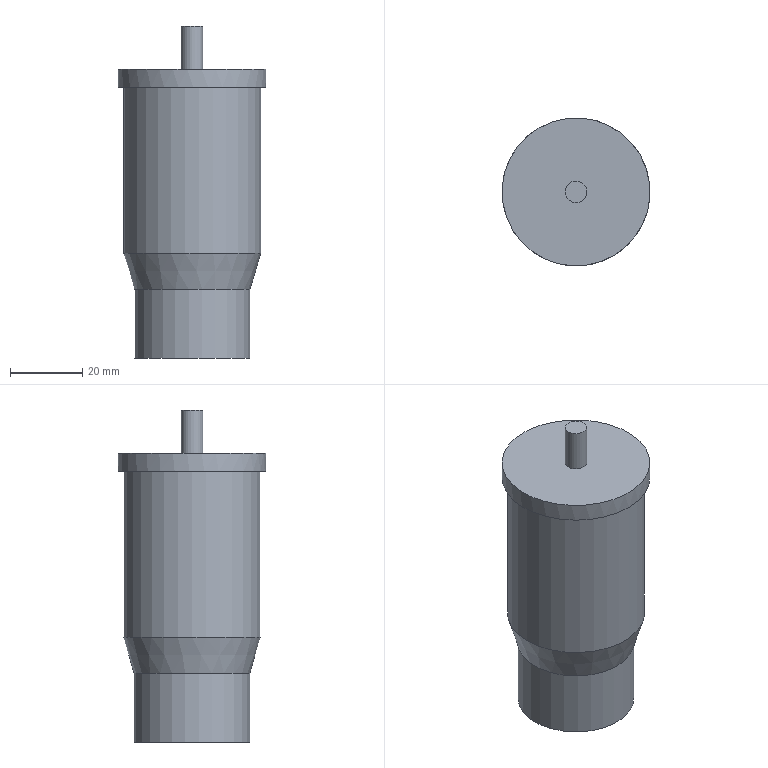Part | NX | features solid 2 | 1 solid | 9 faces | box 41 x 41 x 92 mm | volume 84158 mm3 | plane 4 | cylinder 4 | cone 1 | commonest cylinder face diameters 6 x1 32.1 x1 38 x1 41 x1
STEP:
#1=CARTESIAN_POINT('',(799.065,-200.244,51.));
#2=VERTEX_POINT('',#1);
#3=CARTESIAN_POINT('',(807.09,-214.144,51.));
#4=DIRECTION('',(0.,0.,-1.));
#5=DIRECTION('',(-0.5,0.866,0.));
#6=AXIS2_PLACEMENT_3D('',#3,#4,#5);
#7=CIRCLE('',#6,16.05);
#8=EDGE_CURVE('',#2,#2,#7,.T.);
#9=ORIENTED_EDGE('',*,*,#8,.T.);
#10=EDGE_LOOP('',(#9));
#11=FACE_BOUND('',#10,.T.);
#12=CARTESIAN_POINT('',(807.09,-214.144,51.));
#13=DIRECTION('',(0.,0.,-1.));
#14=DIRECTION('',(0.5,-0.866,0.));
#15=AXIS2_PLACEMENT_3D('',#12,#13,#14);
#16=PLANE('',#15);
#17=ADVANCED_FACE('',(#11),#16,.T.);
#18=CARTESIAN_POINT('',(799.065,-200.244,70.));
#19=VERTEX_POINT('',#18);
#20=CARTESIAN_POINT('',(807.09,-214.144,70.));
#21=DIRECTION('',(0.,0.,-1.));
#22=DIRECTION('',(-0.5,0.866,0.));
#23=AXIS2_PLACEMENT_3D('',#20,#21,#22);
#24=CIRCLE('',#23,16.05);
#25=EDGE_CURVE('',#19,#19,#24,.T.);
#26=ORIENTED_EDGE('',*,*,#25,.T.);
#27=EDGE_LOOP('',(#26));
#28=FACE_BOUND('',#27,.T.);
#29=ORIENTED_EDGE('',*,*,#8,.F.);
#30=EDGE_LOOP('',(#29));
#31=FACE_BOUND('',#30,.T.);
#32=CARTESIAN_POINT('',(807.09,-214.144,51.));
#33=DIRECTION('',(0.,0.,1.));
#34=DIRECTION('',(-0.5,0.866,0.));
#35=AXIS2_PLACEMENT_3D('',#32,#33,#34);
#36=CYLINDRICAL_SURFACE('',#35,16.05);
#37=ADVANCED_FACE('',(#28,#31),#36,.T.);
#38=ORIENTED_EDGE('',*,*,#25,.F.);
#39=EDGE_LOOP('',(#38));
#40=FACE_BOUND('',#39,.T.);
#41=CARTESIAN_POINT('',(797.59,-197.689,80.));
#42=VERTEX_POINT('',#41);
#43=CARTESIAN_POINT('',(807.09,-214.144,80.));
#44=DIRECTION('',(0.,0.,-1.));
#45=DIRECTION('',(-0.5,0.866,0.));
#46=AXIS2_PLACEMENT_3D('',#43,#44,#45);
#47=CIRCLE('',#46,19.);
#48=EDGE_CURVE('',#42,#42,#47,.T.);
#49=ORIENTED_EDGE('',*,*,#48,.T.);
#50=EDGE_LOOP('',(#49));
#51=FACE_BOUND('',#50,.T.);
#52=CARTESIAN_POINT('',(807.09,-214.144,70.));
#53=DIRECTION('',(0.,0.,1.));
#54=DIRECTION('',(-0.5,0.866,0.));
#55=AXIS2_PLACEMENT_3D('',#52,#53,#54);
#56=CONICAL_SURFACE('',#55,16.05,0.2869);
#57=ADVANCED_FACE('',(#40,#51),#56,.T.);
#58=CARTESIAN_POINT('',(816.59,-230.598,126.));
#59=VERTEX_POINT('',#58);
#60=CARTESIAN_POINT('',(807.09,-214.144,126.));
#61=DIRECTION('',(0.,0.,1.));
#62=DIRECTION('',(0.5,-0.866,0.));
#63=AXIS2_PLACEMENT_3D('',#60,#61,#62);
#64=CIRCLE('',#63,19.);
#65=EDGE_CURVE('',#59,#59,#64,.F.);
#66=ORIENTED_EDGE('',*,*,#65,.T.);
#67=EDGE_LOOP('',(#66));
#68=FACE_BOUND('',#67,.T.);
#69=ORIENTED_EDGE('',*,*,#48,.F.);
#70=EDGE_LOOP('',(#69));
#71=FACE_BOUND('',#70,.T.);
#72=CARTESIAN_POINT('',(807.09,-214.144,80.));
#73=DIRECTION('',(0.,0.,1.));
#74=DIRECTION('',(-0.5,0.866,0.));
#75=AXIS2_PLACEMENT_3D('',#72,#73,#74);
#76=CYLINDRICAL_SURFACE('',#75,19.);
#77=ADVANCED_FACE('',(#68,#71),#76,.T.);
#78=CARTESIAN_POINT('',(805.59,-211.545,131.));
#79=VERTEX_POINT('',#78);
#80=CARTESIAN_POINT('',(807.09,-214.144,131.));
#81=DIRECTION('',(0.,0.,-1.));
#82=DIRECTION('',(-0.5,0.866,0.));
#83=AXIS2_PLACEMENT_3D('',#80,#81,#82);
#84=CIRCLE('',#83,3.);
#85=EDGE_CURVE('',#79,#79,#84,.T.);
#86=ORIENTED_EDGE('',*,*,#85,.T.);
#87=EDGE_LOOP('',(#86));
#88=FACE_BOUND('',#87,.T.);
#89=CARTESIAN_POINT('',(817.34,-231.897,131.));
#90=VERTEX_POINT('',#89);
#91=CARTESIAN_POINT('',(807.09,-214.144,131.));
#92=DIRECTION('',(0.,0.,1.));
#93=DIRECTION('',(0.5,-0.866,0.));
#94=AXIS2_PLACEMENT_3D('',#91,#92,#93);
#95=CIRCLE('',#94,20.5);
#96=EDGE_CURVE('',#90,#90,#95,.T.);
#97=ORIENTED_EDGE('',*,*,#96,.T.);
#98=EDGE_LOOP('',(#97));
#99=FACE_BOUND('',#98,.T.);
#100=CARTESIAN_POINT('',(807.09,-214.144,131.));
#101=DIRECTION('',(0.,0.,1.));
#102=DIRECTION('',(-0.5,0.866,0.));
#103=AXIS2_PLACEMENT_3D('',#100,#101,#102);
#104=PLANE('',#103);
#105=ADVANCED_FACE('',(#88,#99),#104,.T.);
#106=ORIENTED_EDGE('',*,*,#65,.F.);
#107=EDGE_LOOP('',(#106));
#108=FACE_BOUND('',#107,.T.);
#109=CARTESIAN_POINT('',(796.84,-196.39,126.));
#110=VERTEX_POINT('',#109);
#111=CARTESIAN_POINT('',(807.09,-214.144,126.));
#112=DIRECTION('',(0.,0.,-1.));
#113=DIRECTION('',(-0.5,0.866,0.));
#114=AXIS2_PLACEMENT_3D('',#111,#112,#113);
#115=CIRCLE('',#114,20.5);
#116=EDGE_CURVE('',#110,#110,#115,.T.);
#117=ORIENTED_EDGE('',*,*,#116,.T.);
#118=EDGE_LOOP('',(#117));
#119=FACE_BOUND('',#118,.T.);
#120=CARTESIAN_POINT('',(807.09,-214.144,126.));
#121=DIRECTION('',(0.,0.,-1.));
#122=DIRECTION('',(0.5,-0.866,0.));
#123=AXIS2_PLACEMENT_3D('',#120,#121,#122);
#124=PLANE('',#123);
#125=ADVANCED_FACE('',(#108,#119),#124,.T.);
#126=ORIENTED_EDGE('',*,*,#96,.F.);
#127=EDGE_LOOP('',(#126));
#128=FACE_BOUND('',#127,.T.);
#129=ORIENTED_EDGE('',*,*,#116,.F.);
#130=EDGE_LOOP('',(#129));
#131=FACE_BOUND('',#130,.T.);
#132=CARTESIAN_POINT('',(807.09,-214.144,136.));
#133=DIRECTION('',(0.,0.,1.));
#134=DIRECTION('',(-0.5,0.866,0.));
#135=AXIS2_PLACEMENT_3D('',#132,#133,#134);
#136=CYLINDRICAL_SURFACE('',#135,20.5);
#137=ADVANCED_FACE('',(#128,#131),#136,.T.);
#138=CARTESIAN_POINT('',(808.59,-216.742,143.));
#139=VERTEX_POINT('',#138);
#140=CARTESIAN_POINT('',(807.09,-214.144,143.));
#141=DIRECTION('',(0.,0.,1.));
#142=DIRECTION('',(0.5,-0.866,0.));
#143=AXIS2_PLACEMENT_3D('',#140,#141,#142);
#144=CIRCLE('',#143,3.);
#145=EDGE_CURVE('',#139,#139,#144,.T.);
#146=ORIENTED_EDGE('',*,*,#145,.T.);
#147=EDGE_LOOP('',(#146));
#148=FACE_BOUND('',#147,.T.);
#149=CARTESIAN_POINT('',(807.09,-214.144,143.));
#150=DIRECTION('',(0.,0.,1.));
#151=DIRECTION('',(-0.5,0.866,0.));
#152=AXIS2_PLACEMENT_3D('',#149,#150,#151);
#153=PLANE('',#152);
#154=ADVANCED_FACE('',(#148),#153,.T.);
#155=ORIENTED_EDGE('',*,*,#145,.F.);
#156=EDGE_LOOP('',(#155));
#157=FACE_BOUND('',#156,.T.);
#158=ORIENTED_EDGE('',*,*,#85,.F.);
#159=EDGE_LOOP('',(#158));
#160=FACE_BOUND('',#159,.T.);
#161=CARTESIAN_POINT('',(807.09,-214.144,141.));
#162=DIRECTION('',(0.,0.,1.));
#163=DIRECTION('',(-0.5,0.866,0.));
#164=AXIS2_PLACEMENT_3D('',#161,#162,#163);
#165=CYLINDRICAL_SURFACE('',#164,3.);
#166=ADVANCED_FACE('',(#157,#160),#165,.T.);
#167=CLOSED_SHELL('',(#17,#37,#57,#77,#105,#125,#137,#154,#166));
#168=MANIFOLD_SOLID_BREP('',#167);
#169=(LENGTH_UNIT()NAMED_UNIT(*)SI_UNIT(.MILLI.,.METRE.));
#170=UNCERTAINTY_MEASURE_WITH_UNIT(LENGTH_MEASURE(0.00001),#169,'','');
#171=(NAMED_UNIT(*)PLANE_ANGLE_UNIT()SI_UNIT($,.RADIAN.));
#172=(NAMED_UNIT(*)SI_UNIT($,.STERADIAN.)SOLID_ANGLE_UNIT());
#173=(GEOMETRIC_REPRESENTATION_CONTEXT(3)GLOBAL_UNCERTAINTY_ASSIGNED_CONTEXT((#170))GLOBAL_UNIT_ASSIGNED_CONTEXT((#169,#171,#172))REPRESENTATION_CONTEXT('',''));
#174=ADVANCED_BREP_SHAPE_REPRESENTATION('',(#168),#173);